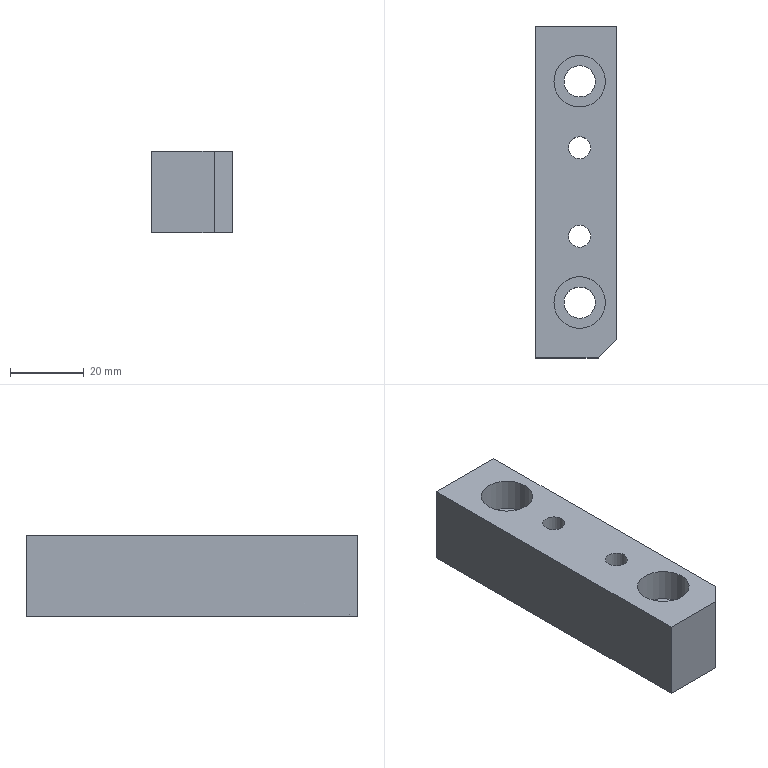Part | STEP file | P011002S004-003 | 1 solid | 15 faces | box 22 x 90 x 22 mm | volume 37795 mm3 | plane 9 | cylinder 6 | commonest cylinder face diameters 6 x2 8.5 x2 14 x2
STEP:
#1=CARTESIAN_POINT('',(0.,0.,0.));
#2=DIRECTION('',(0.,0.,1.));
#3=DIRECTION('',(1.,0.,0.));
#4=AXIS2_PLACEMENT_3D('',#1,#2,#3);
#5=CARTESIAN_POINT('',(90.,-233.,-3.));
#6=VERTEX_POINT('',#5);
#7=CARTESIAN_POINT('',(87.,-233.,-3.));
#8=DIRECTION('',(0.,0.,-1.));
#9=DIRECTION('',(1.,0.,0.));
#10=AXIS2_PLACEMENT_3D('',#7,#8,#9);
#11=CIRCLE('',#10,3.);
#12=CARTESIAN_POINT('',(75.,-258.,-3.));
#13=DIRECTION('',(0.,0.,-1.));
#14=DIRECTION('',(0.,1.,0.));
#15=AXIS2_PLACEMENT_3D('',#12,#13,#14);
#16=PLANE('',#15);
#17=CARTESIAN_POINT('',(25.,12.));
#18=DIRECTION('',(0.,1.));
#19=AXIS2_PLACEMENT_2D('',#17,#18);
#20=CIRCLE('',#19,3.);
#21=(GEOMETRIC_REPRESENTATION_CONTEXT(2)PARAMETRIC_REPRESENTATION_CONTEXT()REPRESENTATION_CONTEXT('',''));
#22=DEFINITIONAL_REPRESENTATION('',(#20),#21);
#23=PCURVE('',#16,#22);
#24=CARTESIAN_POINT('',(87.,-233.,19.));
#25=DIRECTION('',(0.,0.,-1.));
#26=DIRECTION('',(1.,0.,0.));
#27=AXIS2_PLACEMENT_3D('',#24,#25,#26);
#28=CYLINDRICAL_SURFACE('',#27,3.);
#29=CARTESIAN_POINT('',(0.,22.));
#30=DIRECTION('',(1.,0.));
#31=VECTOR('',#30,1.);
#32=LINE('',#29,#31);
#33=(GEOMETRIC_REPRESENTATION_CONTEXT(2)PARAMETRIC_REPRESENTATION_CONTEXT()REPRESENTATION_CONTEXT('',''));
#34=DEFINITIONAL_REPRESENTATION('',(#32),#33);
#35=PCURVE('',#28,#34);
#36=SURFACE_CURVE('',#11,(#23,#35),.PCURVE_S1.);
#37=EDGE_CURVE('',#6,#6,#36,.T.);
#38=ORIENTED_EDGE('',*,*,#37,.F.);
#39=EDGE_LOOP('',(#38));
#40=FACE_BOUND('',#39,.T.);
#41=CARTESIAN_POINT('',(90.,-257.,-3.));
#42=VERTEX_POINT('',#41);
#43=CARTESIAN_POINT('',(87.,-257.,-3.));
#44=DIRECTION('',(0.,0.,-1.));
#45=DIRECTION('',(1.,0.,0.));
#46=AXIS2_PLACEMENT_3D('',#43,#44,#45);
#47=CIRCLE('',#46,3.);
#48=CARTESIAN_POINT('',(1.,12.));
#49=DIRECTION('',(0.,1.));
#50=AXIS2_PLACEMENT_2D('',#48,#49);
#51=CIRCLE('',#50,3.);
#52=(GEOMETRIC_REPRESENTATION_CONTEXT(2)PARAMETRIC_REPRESENTATION_CONTEXT()REPRESENTATION_CONTEXT('',''));
#53=DEFINITIONAL_REPRESENTATION('',(#51),#52);
#54=PCURVE('',#16,#53);
#55=CARTESIAN_POINT('',(87.,-257.,19.));
#56=DIRECTION('',(0.,0.,-1.));
#57=DIRECTION('',(1.,0.,0.));
#58=AXIS2_PLACEMENT_3D('',#55,#56,#57);
#59=CYLINDRICAL_SURFACE('',#58,3.);
#60=CARTESIAN_POINT('',(0.,22.));
#61=DIRECTION('',(1.,0.));
#62=VECTOR('',#61,1.);
#63=LINE('',#60,#62);
#64=(GEOMETRIC_REPRESENTATION_CONTEXT(2)PARAMETRIC_REPRESENTATION_CONTEXT()REPRESENTATION_CONTEXT('',''));
#65=DEFINITIONAL_REPRESENTATION('',(#63),#64);
#66=PCURVE('',#59,#65);
#67=SURFACE_CURVE('',#47,(#54,#66),.PCURVE_S1.);
#68=EDGE_CURVE('',#42,#42,#67,.T.);
#69=ORIENTED_EDGE('',*,*,#68,.F.);
#70=EDGE_LOOP('',(#69));
#71=FACE_BOUND('',#70,.T.);
#72=CARTESIAN_POINT('',(75.,-290.,-3.));
#73=VERTEX_POINT('',#72);
#74=CARTESIAN_POINT('',(92.,-290.,-3.));
#75=VERTEX_POINT('',#74);
#76=CARTESIAN_POINT('',(75.,-290.,-3.));
#77=DIRECTION('',(1.,0.,0.));
#78=VECTOR('',#77,1.);
#79=LINE('',#76,#78);
#80=CARTESIAN_POINT('',(-32.,0.));
#81=DIRECTION('',(0.,1.));
#82=VECTOR('',#81,1.);
#83=LINE('',#80,#82);
#84=(GEOMETRIC_REPRESENTATION_CONTEXT(2)PARAMETRIC_REPRESENTATION_CONTEXT()REPRESENTATION_CONTEXT('',''));
#85=DEFINITIONAL_REPRESENTATION('',(#83),#84);
#86=PCURVE('',#16,#85);
#87=CARTESIAN_POINT('',(-325.,-290.,260.));
#88=DIRECTION('',(0.,1.,0.));
#89=DIRECTION('',(0.,0.,1.));
#90=AXIS2_PLACEMENT_3D('',#87,#88,#89);
#91=PLANE('',#90);
#92=CARTESIAN_POINT('',(-263.,400.));
#93=DIRECTION('',(0.,1.));
#94=VECTOR('',#93,1.);
#95=LINE('',#92,#94);
#96=(GEOMETRIC_REPRESENTATION_CONTEXT(2)PARAMETRIC_REPRESENTATION_CONTEXT()REPRESENTATION_CONTEXT('',''));
#97=DEFINITIONAL_REPRESENTATION('',(#95),#96);
#98=PCURVE('',#91,#97);
#99=SURFACE_CURVE('',#79,(#86,#98),.PCURVE_S1.);
#100=EDGE_CURVE('',#73,#75,#99,.T.);
#101=ORIENTED_EDGE('',*,*,#100,.F.);
#102=CARTESIAN_POINT('',(75.,-200.,-3.));
#103=VERTEX_POINT('',#102);
#104=CARTESIAN_POINT('',(75.,-258.,-3.));
#105=DIRECTION('',(0.,1.,0.));
#106=VECTOR('',#105,1.);
#107=LINE('',#104,#106);
#108=CARTESIAN_POINT('',(0.,0.));
#109=DIRECTION('',(1.,0.));
#110=VECTOR('',#109,1.);
#111=LINE('',#108,#110);
#112=(GEOMETRIC_REPRESENTATION_CONTEXT(2)PARAMETRIC_REPRESENTATION_CONTEXT()REPRESENTATION_CONTEXT('',''));
#113=DEFINITIONAL_REPRESENTATION('',(#111),#112);
#114=PCURVE('',#16,#113);
#115=CARTESIAN_POINT('',(75.,-258.,19.));
#116=DIRECTION('',(-1.,0.,0.));
#117=DIRECTION('',(0.,0.,-1.));
#118=AXIS2_PLACEMENT_3D('',#115,#116,#117);
#119=PLANE('',#118);
#120=CARTESIAN_POINT('',(22.,0.));
#121=DIRECTION('',(0.,-1.));
#122=VECTOR('',#121,1.);
#123=LINE('',#120,#122);
#124=(GEOMETRIC_REPRESENTATION_CONTEXT(2)PARAMETRIC_REPRESENTATION_CONTEXT()REPRESENTATION_CONTEXT('',''));
#125=DEFINITIONAL_REPRESENTATION('',(#123),#124);
#126=PCURVE('',#119,#125);
#127=SURFACE_CURVE('',#107,(#114,#126),.PCURVE_S1.);
#128=EDGE_CURVE('',#73,#103,#127,.T.);
#129=ORIENTED_EDGE('',*,*,#128,.T.);
#130=CARTESIAN_POINT('',(97.,-200.,-3.));
#131=VERTEX_POINT('',#130);
#132=CARTESIAN_POINT('',(-165.,-200.,-3.));
#133=DIRECTION('',(1.,0.,0.));
#134=VECTOR('',#133,1.);
#135=LINE('',#132,#134);
#136=CARTESIAN_POINT('',(58.,-240.));
#137=DIRECTION('',(0.,1.));
#138=VECTOR('',#137,1.);
#139=LINE('',#136,#138);
#140=(GEOMETRIC_REPRESENTATION_CONTEXT(2)PARAMETRIC_REPRESENTATION_CONTEXT()REPRESENTATION_CONTEXT('',''));
#141=DEFINITIONAL_REPRESENTATION('',(#139),#140);
#142=PCURVE('',#16,#141);
#143=CARTESIAN_POINT('',(-165.,-200.,-50.));
#144=DIRECTION('',(0.,-1.,0.));
#145=DIRECTION('',(0.,0.,1.));
#146=AXIS2_PLACEMENT_3D('',#143,#144,#145);
#147=PLANE('',#146);
#148=CARTESIAN_POINT('',(47.,0.));
#149=DIRECTION('',(0.,-1.));
#150=VECTOR('',#149,1.);
#151=LINE('',#148,#150);
#152=(GEOMETRIC_REPRESENTATION_CONTEXT(2)PARAMETRIC_REPRESENTATION_CONTEXT()REPRESENTATION_CONTEXT('',''));
#153=DEFINITIONAL_REPRESENTATION('',(#151),#152);
#154=PCURVE('',#147,#153);
#155=SURFACE_CURVE('',#135,(#142,#154),.PCURVE_S1.);
#156=EDGE_CURVE('',#103,#131,#155,.T.);
#157=ORIENTED_EDGE('',*,*,#156,.T.);
#158=CARTESIAN_POINT('',(97.,-285.,-3.));
#159=VERTEX_POINT('',#158);
#160=CARTESIAN_POINT('',(97.,-258.,-3.));
#161=DIRECTION('',(0.,1.,0.));
#162=VECTOR('',#161,1.);
#163=LINE('',#160,#162);
#164=CARTESIAN_POINT('',(0.,22.));
#165=DIRECTION('',(1.,0.));
#166=VECTOR('',#165,1.);
#167=LINE('',#164,#166);
#168=(GEOMETRIC_REPRESENTATION_CONTEXT(2)PARAMETRIC_REPRESENTATION_CONTEXT()REPRESENTATION_CONTEXT('',''));
#169=DEFINITIONAL_REPRESENTATION('',(#167),#168);
#170=PCURVE('',#16,#169);
#171=CARTESIAN_POINT('',(97.,-258.,19.));
#172=DIRECTION('',(-1.,0.,0.));
#173=DIRECTION('',(0.,0.,-1.));
#174=AXIS2_PLACEMENT_3D('',#171,#172,#173);
#175=PLANE('',#174);
#176=CARTESIAN_POINT('',(22.,0.));
#177=DIRECTION('',(0.,-1.));
#178=VECTOR('',#177,1.);
#179=LINE('',#176,#178);
#180=(GEOMETRIC_REPRESENTATION_CONTEXT(2)PARAMETRIC_REPRESENTATION_CONTEXT()REPRESENTATION_CONTEXT('',''));
#181=DEFINITIONAL_REPRESENTATION('',(#179),#180);
#182=PCURVE('',#175,#181);
#183=SURFACE_CURVE('',#163,(#170,#182),.PCURVE_S1.);
#184=EDGE_CURVE('',#159,#131,#183,.T.);
#185=ORIENTED_EDGE('',*,*,#184,.F.);
#186=CARTESIAN_POINT('',(99.5,-282.5,-3.));
#187=DIRECTION('',(0.7071,0.7071,0.));
#188=VECTOR('',#187,1.);
#189=LINE('',#186,#188);
#190=CARTESIAN_POINT('',(-24.5,24.5));
#191=DIRECTION('',(0.7071,0.7071));
#192=VECTOR('',#191,1.);
#193=LINE('',#190,#192);
#194=(GEOMETRIC_REPRESENTATION_CONTEXT(2)PARAMETRIC_REPRESENTATION_CONTEXT()REPRESENTATION_CONTEXT('',''));
#195=DEFINITIONAL_REPRESENTATION('',(#193),#194);
#196=PCURVE('',#16,#195);
#197=CARTESIAN_POINT('',(97.,-285.,19.));
#198=DIRECTION('',(-0.7071,0.7071,0.));
#199=DIRECTION('',(0.7071,0.7071,0.));
#200=AXIS2_PLACEMENT_3D('',#197,#198,#199);
#201=PLANE('',#200);
#202=CARTESIAN_POINT('',(3.536,22.));
#203=DIRECTION('',(1.,0.));
#204=VECTOR('',#203,1.);
#205=LINE('',#202,#204);
#206=(GEOMETRIC_REPRESENTATION_CONTEXT(2)PARAMETRIC_REPRESENTATION_CONTEXT()REPRESENTATION_CONTEXT('',''));
#207=DEFINITIONAL_REPRESENTATION('',(#205),#206);
#208=PCURVE('',#201,#207);
#209=SURFACE_CURVE('',#189,(#196,#208),.PCURVE_S1.);
#210=EDGE_CURVE('',#75,#159,#209,.T.);
#211=ORIENTED_EDGE('',*,*,#210,.F.);
#212=EDGE_LOOP('',(#101,#129,#157,#185,#211));
#213=FACE_BOUND('',#212,.T.);
#214=CARTESIAN_POINT('',(91.25,-215.,-3.));
#215=VERTEX_POINT('',#214);
#216=CARTESIAN_POINT('',(87.,-215.,-3.));
#217=DIRECTION('',(0.,0.,-1.));
#218=DIRECTION('',(1.,0.,0.));
#219=AXIS2_PLACEMENT_3D('',#216,#217,#218);
#220=CIRCLE('',#219,4.25);
#221=CARTESIAN_POINT('',(43.,12.));
#222=DIRECTION('',(0.,1.));
#223=AXIS2_PLACEMENT_2D('',#221,#222);
#224=CIRCLE('',#223,4.25);
#225=(GEOMETRIC_REPRESENTATION_CONTEXT(2)PARAMETRIC_REPRESENTATION_CONTEXT()REPRESENTATION_CONTEXT('',''));
#226=DEFINITIONAL_REPRESENTATION('',(#224),#225);
#227=PCURVE('',#16,#226);
#228=CARTESIAN_POINT('',(87.,-215.,19.));
#229=DIRECTION('',(0.,0.,-1.));
#230=DIRECTION('',(1.,0.,0.));
#231=AXIS2_PLACEMENT_3D('',#228,#229,#230);
#232=CYLINDRICAL_SURFACE('',#231,4.25);
#233=CARTESIAN_POINT('',(0.,22.));
#234=DIRECTION('',(1.,0.));
#235=VECTOR('',#234,1.);
#236=LINE('',#233,#235);
#237=(GEOMETRIC_REPRESENTATION_CONTEXT(2)PARAMETRIC_REPRESENTATION_CONTEXT()REPRESENTATION_CONTEXT('',''));
#238=DEFINITIONAL_REPRESENTATION('',(#236),#237);
#239=PCURVE('',#232,#238);
#240=SURFACE_CURVE('',#220,(#227,#239),.PCURVE_S1.);
#241=EDGE_CURVE('',#215,#215,#240,.T.);
#242=ORIENTED_EDGE('',*,*,#241,.F.);
#243=EDGE_LOOP('',(#242));
#244=FACE_BOUND('',#243,.T.);
#245=CARTESIAN_POINT('',(91.25,-275.,-3.));
#246=VERTEX_POINT('',#245);
#247=CARTESIAN_POINT('',(87.,-275.,-3.));
#248=DIRECTION('',(0.,0.,-1.));
#249=DIRECTION('',(1.,0.,0.));
#250=AXIS2_PLACEMENT_3D('',#247,#248,#249);
#251=CIRCLE('',#250,4.25);
#252=CARTESIAN_POINT('',(-17.,12.));
#253=DIRECTION('',(0.,1.));
#254=AXIS2_PLACEMENT_2D('',#252,#253);
#255=CIRCLE('',#254,4.25);
#256=(GEOMETRIC_REPRESENTATION_CONTEXT(2)PARAMETRIC_REPRESENTATION_CONTEXT()REPRESENTATION_CONTEXT('',''));
#257=DEFINITIONAL_REPRESENTATION('',(#255),#256);
#258=PCURVE('',#16,#257);
#259=CARTESIAN_POINT('',(87.,-275.,19.));
#260=DIRECTION('',(0.,0.,-1.));
#261=DIRECTION('',(1.,0.,0.));
#262=AXIS2_PLACEMENT_3D('',#259,#260,#261);
#263=CYLINDRICAL_SURFACE('',#262,4.25);
#264=CARTESIAN_POINT('',(0.,22.));
#265=DIRECTION('',(1.,0.));
#266=VECTOR('',#265,1.);
#267=LINE('',#264,#266);
#268=(GEOMETRIC_REPRESENTATION_CONTEXT(2)PARAMETRIC_REPRESENTATION_CONTEXT()REPRESENTATION_CONTEXT('',''));
#269=DEFINITIONAL_REPRESENTATION('',(#267),#268);
#270=PCURVE('',#263,#269);
#271=SURFACE_CURVE('',#251,(#258,#270),.PCURVE_S1.);
#272=EDGE_CURVE('',#246,#246,#271,.T.);
#273=ORIENTED_EDGE('',*,*,#272,.F.);
#274=EDGE_LOOP('',(#273));
#275=FACE_BOUND('',#274,.T.);
#276=ADVANCED_FACE('',(#40,#71,#213,#244,#275),#16,.T.);
#277=CARTESIAN_POINT('',(75.,-290.,19.));
#278=VERTEX_POINT('',#277);
#279=CARTESIAN_POINT('',(92.,-290.,19.));
#280=VERTEX_POINT('',#279);
#281=CARTESIAN_POINT('',(-325.,-290.,19.));
#282=DIRECTION('',(1.,0.,0.));
#283=VECTOR('',#282,1.);
#284=LINE('',#281,#283);
#285=CARTESIAN_POINT('',(-241.,0.));
#286=DIRECTION('',(0.,1.));
#287=VECTOR('',#286,1.);
#288=LINE('',#285,#287);
#289=(GEOMETRIC_REPRESENTATION_CONTEXT(2)PARAMETRIC_REPRESENTATION_CONTEXT()REPRESENTATION_CONTEXT('',''));
#290=DEFINITIONAL_REPRESENTATION('',(#288),#289);
#291=PCURVE('',#91,#290);
#292=CARTESIAN_POINT('',(-275.,-325.,19.));
#293=DIRECTION('',(0.,0.,1.));
#294=DIRECTION('',(-1.,0.,0.));
#295=AXIS2_PLACEMENT_3D('',#292,#293,#294);
#296=PLANE('',#295);
#297=CARTESIAN_POINT('',(50.,-35.));
#298=DIRECTION('',(-1.,0.));
#299=VECTOR('',#298,1.);
#300=LINE('',#297,#299);
#301=(GEOMETRIC_REPRESENTATION_CONTEXT(2)PARAMETRIC_REPRESENTATION_CONTEXT()REPRESENTATION_CONTEXT('',''));
#302=DEFINITIONAL_REPRESENTATION('',(#300),#301);
#303=PCURVE('',#296,#302);
#304=SURFACE_CURVE('',#284,(#291,#303),.PCURVE_S1.);
#305=EDGE_CURVE('',#278,#280,#304,.T.);
#306=ORIENTED_EDGE('',*,*,#305,.F.);
#307=CARTESIAN_POINT('',(75.,-290.,260.));
#308=DIRECTION('',(0.,0.,1.));
#309=VECTOR('',#308,1.);
#310=LINE('',#307,#309);
#311=CARTESIAN_POINT('',(0.,400.));
#312=DIRECTION('',(1.,0.));
#313=VECTOR('',#312,1.);
#314=LINE('',#311,#313);
#315=(GEOMETRIC_REPRESENTATION_CONTEXT(2)PARAMETRIC_REPRESENTATION_CONTEXT()REPRESENTATION_CONTEXT('',''));
#316=DEFINITIONAL_REPRESENTATION('',(#314),#315);
#317=PCURVE('',#91,#316);
#318=CARTESIAN_POINT('',(-241.,32.));
#319=DIRECTION('',(-1.,0.));
#320=VECTOR('',#319,1.);
#321=LINE('',#318,#320);
#322=(GEOMETRIC_REPRESENTATION_CONTEXT(2)PARAMETRIC_REPRESENTATION_CONTEXT()REPRESENTATION_CONTEXT('',''));
#323=DEFINITIONAL_REPRESENTATION('',(#321),#322);
#324=PCURVE('',#119,#323);
#325=SURFACE_CURVE('',#310,(#317,#324),.PCURVE_S1.);
#326=EDGE_CURVE('',#73,#278,#325,.T.);
#327=ORIENTED_EDGE('',*,*,#326,.F.);
#328=ORIENTED_EDGE('',*,*,#100,.T.);
#329=CARTESIAN_POINT('',(92.,-290.,-3.));
#330=DIRECTION('',(0.,0.,-1.));
#331=VECTOR('',#330,1.);
#332=LINE('',#329,#331);
#333=CARTESIAN_POINT('',(-263.,417.));
#334=DIRECTION('',(-1.,0.));
#335=VECTOR('',#334,1.);
#336=LINE('',#333,#335);
#337=(GEOMETRIC_REPRESENTATION_CONTEXT(2)PARAMETRIC_REPRESENTATION_CONTEXT()REPRESENTATION_CONTEXT('',''));
#338=DEFINITIONAL_REPRESENTATION('',(#336),#337);
#339=PCURVE('',#91,#338);
#340=CARTESIAN_POINT('',(-7.071,22.));
#341=DIRECTION('',(0.,1.));
#342=VECTOR('',#341,1.);
#343=LINE('',#340,#342);
#344=(GEOMETRIC_REPRESENTATION_CONTEXT(2)PARAMETRIC_REPRESENTATION_CONTEXT()REPRESENTATION_CONTEXT('',''));
#345=DEFINITIONAL_REPRESENTATION('',(#343),#344);
#346=PCURVE('',#201,#345);
#347=SURFACE_CURVE('',#332,(#339,#346),.PCURVE_S1.);
#348=EDGE_CURVE('',#280,#75,#347,.T.);
#349=ORIENTED_EDGE('',*,*,#348,.F.);
#350=EDGE_LOOP('',(#306,#327,#328,#349));
#351=FACE_BOUND('',#350,.T.);
#352=ADVANCED_FACE('',(#351),#91,.F.);
#353=CARTESIAN_POINT('',(80.,-275.,19.));
#354=VERTEX_POINT('',#353);
#355=CARTESIAN_POINT('',(87.,-275.,19.));
#356=DIRECTION('',(0.,0.,-1.));
#357=DIRECTION('',(-1.,0.,0.));
#358=AXIS2_PLACEMENT_3D('',#355,#356,#357);
#359=CIRCLE('',#358,7.);
#360=CARTESIAN_POINT('',(-355.,-50.));
#361=CARTESIAN_POINT('',(-355.,-62.124));
#362=CARTESIAN_POINT('',(-365.5,-56.062));
#363=CARTESIAN_POINT('',(-376.,-50.));
#364=CARTESIAN_POINT('',(-365.5,-43.938));
#365=CARTESIAN_POINT('',(-355.,-37.876));
#366=CARTESIAN_POINT('',(-355.,-50.));
#367=(BOUNDED_CURVE()B_SPLINE_CURVE(2,(#360,#361,#362,#363,#364,#365,#366),.UNSPECIFIED.,.T.,.F.)B_SPLINE_CURVE_WITH_KNOTS((1,2,2,2,2,1),(-2.094,0.,2.094,4.189,6.283,8.378),.UNSPECIFIED.)CURVE()GEOMETRIC_REPRESENTATION_ITEM()RATIONAL_B_SPLINE_CURVE((1.,0.5,1.,0.5,1.,0.5,1.))REPRESENTATION_ITEM(''));
#368=(GEOMETRIC_REPRESENTATION_CONTEXT(2)PARAMETRIC_REPRESENTATION_CONTEXT()REPRESENTATION_CONTEXT('',''));
#369=DEFINITIONAL_REPRESENTATION('',(#367),#368);
#370=PCURVE('',#296,#369);
#371=CARTESIAN_POINT('',(87.,-275.,19.));
#372=DIRECTION('',(0.,0.,-1.));
#373=DIRECTION('',(1.,0.,0.));
#374=AXIS2_PLACEMENT_3D('',#371,#372,#373);
#375=CYLINDRICAL_SURFACE('',#374,7.);
#376=CARTESIAN_POINT('',(3.142,0.));
#377=DIRECTION('',(1.,0.));
#378=VECTOR('',#377,1.);
#379=LINE('',#376,#378);
#380=(GEOMETRIC_REPRESENTATION_CONTEXT(2)PARAMETRIC_REPRESENTATION_CONTEXT()REPRESENTATION_CONTEXT('',''));
#381=DEFINITIONAL_REPRESENTATION('',(#379),#380);
#382=PCURVE('',#375,#381);
#383=SURFACE_CURVE('',#359,(#370,#382),.PCURVE_S1.);
#384=EDGE_CURVE('',#354,#354,#383,.T.);
#385=ORIENTED_EDGE('',*,*,#384,.T.);
#386=EDGE_LOOP('',(#385));
#387=FACE_BOUND('',#386,.T.);
#388=CARTESIAN_POINT('',(84.,-233.,19.));
#389=VERTEX_POINT('',#388);
#390=CARTESIAN_POINT('',(90.,-233.,19.));
#391=VERTEX_POINT('',#390);
#392=CARTESIAN_POINT('',(87.,-233.,19.));
#393=DIRECTION('',(0.,0.,-1.));
#394=DIRECTION('',(-1.,0.,0.));
#395=AXIS2_PLACEMENT_3D('',#392,#393,#394);
#396=CIRCLE('',#395,3.);
#397=CARTESIAN_POINT('',(-359.,-92.));
#398=CARTESIAN_POINT('',(-359.,-97.196));
#399=CARTESIAN_POINT('',(-363.5,-94.598));
#400=CARTESIAN_POINT('',(-368.,-92.));
#401=CARTESIAN_POINT('',(-363.5,-89.402));
#402=CARTESIAN_POINT('',(-359.,-86.804));
#403=CARTESIAN_POINT('',(-359.,-92.));
#404=(BOUNDED_CURVE()B_SPLINE_CURVE(2,(#397,#398,#399,#400,#401,#402,#403),.UNSPECIFIED.,.T.,.F.)B_SPLINE_CURVE_WITH_KNOTS((1,2,2,2,2,1),(-2.094,0.,2.094,4.189,6.283,8.378),.UNSPECIFIED.)CURVE()GEOMETRIC_REPRESENTATION_ITEM()RATIONAL_B_SPLINE_CURVE((1.,0.5,1.,0.5,1.,0.5,1.))REPRESENTATION_ITEM(''));
#405=(GEOMETRIC_REPRESENTATION_CONTEXT(2)PARAMETRIC_REPRESENTATION_CONTEXT()REPRESENTATION_CONTEXT('',''));
#406=DEFINITIONAL_REPRESENTATION('',(#404),#405);
#407=PCURVE('',#296,#406);
#408=CARTESIAN_POINT('',(3.142,0.));
#409=DIRECTION('',(1.,0.));
#410=VECTOR('',#409,1.);
#411=LINE('',#408,#410);
#412=(GEOMETRIC_REPRESENTATION_CONTEXT(2)PARAMETRIC_REPRESENTATION_CONTEXT()REPRESENTATION_CONTEXT('',''));
#413=DEFINITIONAL_REPRESENTATION('',(#411),#412);
#414=PCURVE('',#28,#413);
#415=SURFACE_CURVE('',#396,(#407,#414),.PCURVE_S1.);
#416=EDGE_CURVE('',#389,#391,#415,.T.);
#417=ORIENTED_EDGE('',*,*,#416,.T.);
#418=CARTESIAN_POINT('',(87.,-233.,19.));
#419=DIRECTION('',(0.,0.,-1.));
#420=DIRECTION('',(-1.,0.,0.));
#421=AXIS2_PLACEMENT_3D('',#418,#419,#420);
#422=CIRCLE('',#421,3.);
#423=CARTESIAN_POINT('',(-359.,-92.));
#424=CARTESIAN_POINT('',(-359.,-97.196));
#425=CARTESIAN_POINT('',(-363.5,-94.598));
#426=CARTESIAN_POINT('',(-368.,-92.));
#427=CARTESIAN_POINT('',(-363.5,-89.402));
#428=CARTESIAN_POINT('',(-359.,-86.804));
#429=CARTESIAN_POINT('',(-359.,-92.));
#430=(BOUNDED_CURVE()B_SPLINE_CURVE(2,(#423,#424,#425,#426,#427,#428,#429),.UNSPECIFIED.,.T.,.F.)B_SPLINE_CURVE_WITH_KNOTS((1,2,2,2,2,1),(-2.094,0.,2.094,4.189,6.283,8.378),.UNSPECIFIED.)CURVE()GEOMETRIC_REPRESENTATION_ITEM()RATIONAL_B_SPLINE_CURVE((1.,0.5,1.,0.5,1.,0.5,1.))REPRESENTATION_ITEM(''));
#431=(GEOMETRIC_REPRESENTATION_CONTEXT(2)PARAMETRIC_REPRESENTATION_CONTEXT()REPRESENTATION_CONTEXT('',''));
#432=DEFINITIONAL_REPRESENTATION('',(#430),#431);
#433=PCURVE('',#296,#432);
#434=CARTESIAN_POINT('',(-3.142,0.));
#435=DIRECTION('',(1.,0.));
#436=VECTOR('',#435,1.);
#437=LINE('',#434,#436);
#438=(GEOMETRIC_REPRESENTATION_CONTEXT(2)PARAMETRIC_REPRESENTATION_CONTEXT()REPRESENTATION_CONTEXT('',''));
#439=DEFINITIONAL_REPRESENTATION('',(#437),#438);
#440=PCURVE('',#28,#439);
#441=SURFACE_CURVE('',#422,(#433,#440),.PCURVE_S1.);
#442=EDGE_CURVE('',#391,#389,#441,.T.);
#443=ORIENTED_EDGE('',*,*,#442,.T.);
#444=EDGE_LOOP('',(#417,#443));
#445=FACE_BOUND('',#444,.T.);
#446=CARTESIAN_POINT('',(80.,-215.,19.));
#447=VERTEX_POINT('',#446);
#448=CARTESIAN_POINT('',(87.,-215.,19.));
#449=DIRECTION('',(0.,0.,-1.));
#450=DIRECTION('',(-1.,0.,0.));
#451=AXIS2_PLACEMENT_3D('',#448,#449,#450);
#452=CIRCLE('',#451,7.);
#453=CARTESIAN_POINT('',(-355.,-110.));
#454=CARTESIAN_POINT('',(-355.,-122.124));
#455=CARTESIAN_POINT('',(-365.5,-116.062));
#456=CARTESIAN_POINT('',(-376.,-110.));
#457=CARTESIAN_POINT('',(-365.5,-103.938));
#458=CARTESIAN_POINT('',(-355.,-97.876));
#459=CARTESIAN_POINT('',(-355.,-110.));
#460=(BOUNDED_CURVE()B_SPLINE_CURVE(2,(#453,#454,#455,#456,#457,#458,#459),.UNSPECIFIED.,.T.,.F.)B_SPLINE_CURVE_WITH_KNOTS((1,2,2,2,2,1),(-2.094,0.,2.094,4.189,6.283,8.378),.UNSPECIFIED.)CURVE()GEOMETRIC_REPRESENTATION_ITEM()RATIONAL_B_SPLINE_CURVE((1.,0.5,1.,0.5,1.,0.5,1.))REPRESENTATION_ITEM(''));
#461=(GEOMETRIC_REPRESENTATION_CONTEXT(2)PARAMETRIC_REPRESENTATION_CONTEXT()REPRESENTATION_CONTEXT('',''));
#462=DEFINITIONAL_REPRESENTATION('',(#460),#461);
#463=PCURVE('',#296,#462);
#464=CARTESIAN_POINT('',(87.,-215.,19.));
#465=DIRECTION('',(0.,0.,-1.));
#466=DIRECTION('',(1.,0.,0.));
#467=AXIS2_PLACEMENT_3D('',#464,#465,#466);
#468=CYLINDRICAL_SURFACE('',#467,7.);
#469=CARTESIAN_POINT('',(3.142,0.));
#470=DIRECTION('',(1.,0.));
#471=VECTOR('',#470,1.);
#472=LINE('',#469,#471);
#473=(GEOMETRIC_REPRESENTATION_CONTEXT(2)PARAMETRIC_REPRESENTATION_CONTEXT()REPRESENTATION_CONTEXT('',''));
#474=DEFINITIONAL_REPRESENTATION('',(#472),#473);
#475=PCURVE('',#468,#474);
#476=SURFACE_CURVE('',#452,(#463,#475),.PCURVE_S1.);
#477=EDGE_CURVE('',#447,#447,#476,.T.);
#478=ORIENTED_EDGE('',*,*,#477,.T.);
#479=EDGE_LOOP('',(#478));
#480=FACE_BOUND('',#479,.T.);
#481=CARTESIAN_POINT('',(84.,-257.,19.));
#482=VERTEX_POINT('',#481);
#483=CARTESIAN_POINT('',(90.,-257.,19.));
#484=VERTEX_POINT('',#483);
#485=CARTESIAN_POINT('',(87.,-257.,19.));
#486=DIRECTION('',(0.,0.,-1.));
#487=DIRECTION('',(-1.,0.,0.));
#488=AXIS2_PLACEMENT_3D('',#485,#486,#487);
#489=CIRCLE('',#488,3.);
#490=CARTESIAN_POINT('',(-359.,-68.));
#491=CARTESIAN_POINT('',(-359.,-73.196));
#492=CARTESIAN_POINT('',(-363.5,-70.598));
#493=CARTESIAN_POINT('',(-368.,-68.));
#494=CARTESIAN_POINT('',(-363.5,-65.402));
#495=CARTESIAN_POINT('',(-359.,-62.804));
#496=CARTESIAN_POINT('',(-359.,-68.));
#497=(BOUNDED_CURVE()B_SPLINE_CURVE(2,(#490,#491,#492,#493,#494,#495,#496),.UNSPECIFIED.,.T.,.F.)B_SPLINE_CURVE_WITH_KNOTS((1,2,2,2,2,1),(-2.094,0.,2.094,4.189,6.283,8.378),.UNSPECIFIED.)CURVE()GEOMETRIC_REPRESENTATION_ITEM()RATIONAL_B_SPLINE_CURVE((1.,0.5,1.,0.5,1.,0.5,1.))REPRESENTATION_ITEM(''));
#498=(GEOMETRIC_REPRESENTATION_CONTEXT(2)PARAMETRIC_REPRESENTATION_CONTEXT()REPRESENTATION_CONTEXT('',''));
#499=DEFINITIONAL_REPRESENTATION('',(#497),#498);
#500=PCURVE('',#296,#499);
#501=CARTESIAN_POINT('',(3.142,0.));
#502=DIRECTION('',(1.,0.));
#503=VECTOR('',#502,1.);
#504=LINE('',#501,#503);
#505=(GEOMETRIC_REPRESENTATION_CONTEXT(2)PARAMETRIC_REPRESENTATION_CONTEXT()REPRESENTATION_CONTEXT('',''));
#506=DEFINITIONAL_REPRESENTATION('',(#504),#505);
#507=PCURVE('',#59,#506);
#508=SURFACE_CURVE('',#489,(#500,#507),.PCURVE_S1.);
#509=EDGE_CURVE('',#482,#484,#508,.T.);
#510=ORIENTED_EDGE('',*,*,#509,.T.);
#511=CARTESIAN_POINT('',(87.,-257.,19.));
#512=DIRECTION('',(0.,0.,-1.));
#513=DIRECTION('',(-1.,0.,0.));
#514=AXIS2_PLACEMENT_3D('',#511,#512,#513);
#515=CIRCLE('',#514,3.);
#516=CARTESIAN_POINT('',(-359.,-68.));
#517=CARTESIAN_POINT('',(-359.,-73.196));
#518=CARTESIAN_POINT('',(-363.5,-70.598));
#519=CARTESIAN_POINT('',(-368.,-68.));
#520=CARTESIAN_POINT('',(-363.5,-65.402));
#521=CARTESIAN_POINT('',(-359.,-62.804));
#522=CARTESIAN_POINT('',(-359.,-68.));
#523=(BOUNDED_CURVE()B_SPLINE_CURVE(2,(#516,#517,#518,#519,#520,#521,#522),.UNSPECIFIED.,.T.,.F.)B_SPLINE_CURVE_WITH_KNOTS((1,2,2,2,2,1),(-2.094,0.,2.094,4.189,6.283,8.378),.UNSPECIFIED.)CURVE()GEOMETRIC_REPRESENTATION_ITEM()RATIONAL_B_SPLINE_CURVE((1.,0.5,1.,0.5,1.,0.5,1.))REPRESENTATION_ITEM(''));
#524=(GEOMETRIC_REPRESENTATION_CONTEXT(2)PARAMETRIC_REPRESENTATION_CONTEXT()REPRESENTATION_CONTEXT('',''));
#525=DEFINITIONAL_REPRESENTATION('',(#523),#524);
#526=PCURVE('',#296,#525);
#527=CARTESIAN_POINT('',(-3.142,0.));
#528=DIRECTION('',(1.,0.));
#529=VECTOR('',#528,1.);
#530=LINE('',#527,#529);
#531=(GEOMETRIC_REPRESENTATION_CONTEXT(2)PARAMETRIC_REPRESENTATION_CONTEXT()REPRESENTATION_CONTEXT('',''));
#532=DEFINITIONAL_REPRESENTATION('',(#530),#531);
#533=PCURVE('',#59,#532);
#534=SURFACE_CURVE('',#515,(#526,#533),.PCURVE_S1.);
#535=EDGE_CURVE('',#484,#482,#534,.T.);
#536=ORIENTED_EDGE('',*,*,#535,.T.);
#537=EDGE_LOOP('',(#510,#536));
#538=FACE_BOUND('',#537,.T.);
#539=CARTESIAN_POINT('',(97.,-285.,19.));
#540=VERTEX_POINT('',#539);
#541=CARTESIAN_POINT('',(97.,-200.,19.));
#542=VERTEX_POINT('',#541);
#543=CARTESIAN_POINT('',(97.,-325.,19.));
#544=DIRECTION('',(0.,1.,0.));
#545=VECTOR('',#544,1.);
#546=LINE('',#543,#545);
#547=CARTESIAN_POINT('',(-372.,0.));
#548=DIRECTION('',(0.,-1.));
#549=VECTOR('',#548,1.);
#550=LINE('',#547,#549);
#551=(GEOMETRIC_REPRESENTATION_CONTEXT(2)PARAMETRIC_REPRESENTATION_CONTEXT()REPRESENTATION_CONTEXT('',''));
#552=DEFINITIONAL_REPRESENTATION('',(#550),#551);
#553=PCURVE('',#296,#552);
#554=CARTESIAN_POINT('',(0.,67.));
#555=DIRECTION('',(0.,-1.));
#556=VECTOR('',#555,1.);
#557=LINE('',#554,#556);
#558=(GEOMETRIC_REPRESENTATION_CONTEXT(2)PARAMETRIC_REPRESENTATION_CONTEXT()REPRESENTATION_CONTEXT('',''));
#559=DEFINITIONAL_REPRESENTATION('',(#557),#558);
#560=PCURVE('',#175,#559);
#561=SURFACE_CURVE('',#546,(#553,#560),.PCURVE_S1.);
#562=EDGE_CURVE('',#540,#542,#561,.T.);
#563=ORIENTED_EDGE('',*,*,#562,.T.);
#564=CARTESIAN_POINT('',(75.,-200.,19.));
#565=VERTEX_POINT('',#564);
#566=CARTESIAN_POINT('',(-275.,-200.,19.));
#567=DIRECTION('',(1.,0.,0.));
#568=VECTOR('',#567,1.);
#569=LINE('',#566,#568);
#570=CARTESIAN_POINT('',(0.,-125.));
#571=DIRECTION('',(-1.,0.));
#572=VECTOR('',#571,1.);
#573=LINE('',#570,#572);
#574=(GEOMETRIC_REPRESENTATION_CONTEXT(2)PARAMETRIC_REPRESENTATION_CONTEXT()REPRESENTATION_CONTEXT('',''));
#575=DEFINITIONAL_REPRESENTATION('',(#573),#574);
#576=PCURVE('',#296,#575);
#577=CARTESIAN_POINT('',(69.,110.));
#578=DIRECTION('',(0.,-1.));
#579=VECTOR('',#578,1.);
#580=LINE('',#577,#579);
#581=(GEOMETRIC_REPRESENTATION_CONTEXT(2)PARAMETRIC_REPRESENTATION_CONTEXT()REPRESENTATION_CONTEXT('',''));
#582=DEFINITIONAL_REPRESENTATION('',(#580),#581);
#583=PCURVE('',#147,#582);
#584=SURFACE_CURVE('',#569,(#576,#583),.PCURVE_S1.);
#585=EDGE_CURVE('',#565,#542,#584,.T.);
#586=ORIENTED_EDGE('',*,*,#585,.F.);
#587=CARTESIAN_POINT('',(75.,-325.,19.));
#588=DIRECTION('',(0.,1.,0.));
#589=VECTOR('',#588,1.);
#590=LINE('',#587,#589);
#591=CARTESIAN_POINT('',(-350.,0.));
#592=DIRECTION('',(0.,-1.));
#593=VECTOR('',#592,1.);
#594=LINE('',#591,#593);
#595=(GEOMETRIC_REPRESENTATION_CONTEXT(2)PARAMETRIC_REPRESENTATION_CONTEXT()REPRESENTATION_CONTEXT('',''));
#596=DEFINITIONAL_REPRESENTATION('',(#594),#595);
#597=PCURVE('',#296,#596);
#598=CARTESIAN_POINT('',(0.,67.));
#599=DIRECTION('',(0.,-1.));
#600=VECTOR('',#599,1.);
#601=LINE('',#598,#600);
#602=(GEOMETRIC_REPRESENTATION_CONTEXT(2)PARAMETRIC_REPRESENTATION_CONTEXT()REPRESENTATION_CONTEXT('',''));
#603=DEFINITIONAL_REPRESENTATION('',(#601),#602);
#604=PCURVE('',#119,#603);
#605=SURFACE_CURVE('',#590,(#597,#604),.PCURVE_S1.);
#606=EDGE_CURVE('',#278,#565,#605,.T.);
#607=ORIENTED_EDGE('',*,*,#606,.F.);
#608=ORIENTED_EDGE('',*,*,#305,.T.);
#609=CARTESIAN_POINT('',(-109.,-491.,19.));
#610=DIRECTION('',(-0.7071,-0.7071,0.));
#611=VECTOR('',#610,1.);
#612=LINE('',#609,#611);
#613=CARTESIAN_POINT('',(-166.,166.));
#614=DIRECTION('',(0.7071,0.7071));
#615=VECTOR('',#614,1.);
#616=LINE('',#613,#615);
#617=(GEOMETRIC_REPRESENTATION_CONTEXT(2)PARAMETRIC_REPRESENTATION_CONTEXT()REPRESENTATION_CONTEXT('',''));
#618=DEFINITIONAL_REPRESENTATION('',(#616),#617);
#619=PCURVE('',#296,#618);
#620=CARTESIAN_POINT('',(-291.328,0.));
#621=DIRECTION('',(-1.,0.));
#622=VECTOR('',#621,1.);
#623=LINE('',#620,#622);
#624=(GEOMETRIC_REPRESENTATION_CONTEXT(2)PARAMETRIC_REPRESENTATION_CONTEXT()REPRESENTATION_CONTEXT('',''));
#625=DEFINITIONAL_REPRESENTATION('',(#623),#624);
#626=PCURVE('',#201,#625);
#627=SURFACE_CURVE('',#612,(#619,#626),.PCURVE_S1.);
#628=EDGE_CURVE('',#540,#280,#627,.T.);
#629=ORIENTED_EDGE('',*,*,#628,.F.);
#630=EDGE_LOOP('',(#563,#586,#607,#608,#629));
#631=FACE_BOUND('',#630,.T.);
#632=ADVANCED_FACE('',(#387,#445,#480,#538,#631),#296,.T.);
#633=CARTESIAN_POINT('',(75.,-200.,19.));
#634=DIRECTION('',(0.,0.,1.));
#635=VECTOR('',#634,1.);
#636=LINE('',#633,#635);
#637=CARTESIAN_POINT('',(69.,-240.));
#638=DIRECTION('',(1.,0.));
#639=VECTOR('',#638,1.);
#640=LINE('',#637,#639);
#641=(GEOMETRIC_REPRESENTATION_CONTEXT(2)PARAMETRIC_REPRESENTATION_CONTEXT()REPRESENTATION_CONTEXT('',''));
#642=DEFINITIONAL_REPRESENTATION('',(#640),#641);
#643=PCURVE('',#147,#642);
#644=CARTESIAN_POINT('',(0.,-58.));
#645=DIRECTION('',(-1.,0.));
#646=VECTOR('',#645,1.);
#647=LINE('',#644,#646);
#648=(GEOMETRIC_REPRESENTATION_CONTEXT(2)PARAMETRIC_REPRESENTATION_CONTEXT()REPRESENTATION_CONTEXT('',''));
#649=DEFINITIONAL_REPRESENTATION('',(#647),#648);
#650=PCURVE('',#119,#649);
#651=SURFACE_CURVE('',#636,(#643,#650),.PCURVE_S1.);
#652=EDGE_CURVE('',#103,#565,#651,.T.);
#653=ORIENTED_EDGE('',*,*,#652,.T.);
#654=ORIENTED_EDGE('',*,*,#585,.T.);
#655=CARTESIAN_POINT('',(97.,-200.,19.));
#656=DIRECTION('',(0.,0.,1.));
#657=VECTOR('',#656,1.);
#658=LINE('',#655,#657);
#659=CARTESIAN_POINT('',(69.,-262.));
#660=DIRECTION('',(1.,0.));
#661=VECTOR('',#660,1.);
#662=LINE('',#659,#661);
#663=(GEOMETRIC_REPRESENTATION_CONTEXT(2)PARAMETRIC_REPRESENTATION_CONTEXT()REPRESENTATION_CONTEXT('',''));
#664=DEFINITIONAL_REPRESENTATION('',(#662),#663);
#665=PCURVE('',#147,#664);
#666=CARTESIAN_POINT('',(0.,-58.));
#667=DIRECTION('',(-1.,0.));
#668=VECTOR('',#667,1.);
#669=LINE('',#666,#668);
#670=(GEOMETRIC_REPRESENTATION_CONTEXT(2)PARAMETRIC_REPRESENTATION_CONTEXT()REPRESENTATION_CONTEXT('',''));
#671=DEFINITIONAL_REPRESENTATION('',(#669),#670);
#672=PCURVE('',#175,#671);
#673=SURFACE_CURVE('',#658,(#665,#672),.PCURVE_S1.);
#674=EDGE_CURVE('',#131,#542,#673,.T.);
#675=ORIENTED_EDGE('',*,*,#674,.F.);
#676=ORIENTED_EDGE('',*,*,#156,.F.);
#677=EDGE_LOOP('',(#653,#654,#675,#676));
#678=FACE_BOUND('',#677,.T.);
#679=ADVANCED_FACE('',(#678),#147,.F.);
#680=ORIENTED_EDGE('',*,*,#184,.T.);
#681=ORIENTED_EDGE('',*,*,#674,.T.);
#682=ORIENTED_EDGE('',*,*,#562,.F.);
#683=CARTESIAN_POINT('',(97.,-285.,19.));
#684=DIRECTION('',(0.,0.,1.));
#685=VECTOR('',#684,1.);
#686=LINE('',#683,#685);
#687=CARTESIAN_POINT('',(0.,27.));
#688=DIRECTION('',(-1.,0.));
#689=VECTOR('',#688,1.);
#690=LINE('',#687,#689);
#691=(GEOMETRIC_REPRESENTATION_CONTEXT(2)PARAMETRIC_REPRESENTATION_CONTEXT()REPRESENTATION_CONTEXT('',''));
#692=DEFINITIONAL_REPRESENTATION('',(#690),#691);
#693=PCURVE('',#175,#692);
#694=CARTESIAN_POINT('',(0.,0.));
#695=DIRECTION('',(0.,-1.));
#696=VECTOR('',#695,1.);
#697=LINE('',#694,#696);
#698=(GEOMETRIC_REPRESENTATION_CONTEXT(2)PARAMETRIC_REPRESENTATION_CONTEXT()REPRESENTATION_CONTEXT('',''));
#699=DEFINITIONAL_REPRESENTATION('',(#697),#698);
#700=PCURVE('',#201,#699);
#701=SURFACE_CURVE('',#686,(#693,#700),.PCURVE_S1.);
#702=EDGE_CURVE('',#159,#540,#701,.T.);
#703=ORIENTED_EDGE('',*,*,#702,.F.);
#704=EDGE_LOOP('',(#680,#681,#682,#703));
#705=FACE_BOUND('',#704,.T.);
#706=ADVANCED_FACE('',(#705),#175,.F.);
#707=ORIENTED_EDGE('',*,*,#606,.T.);
#708=ORIENTED_EDGE('',*,*,#652,.F.);
#709=ORIENTED_EDGE('',*,*,#128,.F.);
#710=ORIENTED_EDGE('',*,*,#326,.T.);
#711=EDGE_LOOP('',(#707,#708,#709,#710));
#712=FACE_BOUND('',#711,.T.);
#713=ADVANCED_FACE('',(#712),#119,.T.);
#714=ORIENTED_EDGE('',*,*,#210,.T.);
#715=ORIENTED_EDGE('',*,*,#702,.T.);
#716=ORIENTED_EDGE('',*,*,#628,.T.);
#717=ORIENTED_EDGE('',*,*,#348,.T.);
#718=EDGE_LOOP('',(#714,#715,#716,#717));
#719=FACE_BOUND('',#718,.T.);
#720=ADVANCED_FACE('',(#719),#201,.F.);
#721=ORIENTED_EDGE('',*,*,#68,.F.);
#722=CARTESIAN_POINT('',(90.,-257.,19.));
#723=CARTESIAN_POINT('',(90.,-257.,-3.));
#724=B_SPLINE_CURVE_WITH_KNOTS('',1,(#722,#723),.UNSPECIFIED.,.F.,.F.,(2,2),(0.,22.),.PIECEWISE_BEZIER_KNOTS.);
#725=CARTESIAN_POINT('',(0.,0.));
#726=DIRECTION('',(0.,1.));
#727=VECTOR('',#726,1.);
#728=LINE('',#725,#727);
#729=(GEOMETRIC_REPRESENTATION_CONTEXT(2)PARAMETRIC_REPRESENTATION_CONTEXT()REPRESENTATION_CONTEXT('',''));
#730=DEFINITIONAL_REPRESENTATION('',(#728),#729);
#731=PCURVE('',#59,#730);
#732=CARTESIAN_POINT('',(6.283,0.));
#733=DIRECTION('',(0.,1.));
#734=VECTOR('',#733,1.);
#735=LINE('',#732,#734);
#736=(GEOMETRIC_REPRESENTATION_CONTEXT(2)PARAMETRIC_REPRESENTATION_CONTEXT()REPRESENTATION_CONTEXT('',''));
#737=DEFINITIONAL_REPRESENTATION('',(#735),#736);
#738=PCURVE('',#59,#737);
#739=SEAM_CURVE('',#724,(#731,#738),.PCURVE_S1.);
#740=EDGE_CURVE('',#484,#42,#739,.T.);
#741=ORIENTED_EDGE('',*,*,#740,.F.);
#742=ORIENTED_EDGE('',*,*,#535,.T.);
#743=ORIENTED_EDGE('',*,*,#509,.T.);
#744=ORIENTED_EDGE('',*,*,#740,.T.);
#745=EDGE_LOOP('',(#721,#741,#742,#743,#744));
#746=FACE_BOUND('',#745,.F.);
#747=ADVANCED_FACE('',(#746),#59,.F.);
#748=ORIENTED_EDGE('',*,*,#241,.F.);
#749=CARTESIAN_POINT('',(91.25,-215.,10.));
#750=VERTEX_POINT('',#749);
#751=CARTESIAN_POINT('',(91.25,-215.,10.));
#752=CARTESIAN_POINT('',(91.25,-215.,-3.));
#753=B_SPLINE_CURVE_WITH_KNOTS('',1,(#751,#752),.UNSPECIFIED.,.F.,.F.,(2,2),(9.,22.),.PIECEWISE_BEZIER_KNOTS.);
#754=CARTESIAN_POINT('',(0.,0.));
#755=DIRECTION('',(0.,1.));
#756=VECTOR('',#755,1.);
#757=LINE('',#754,#756);
#758=(GEOMETRIC_REPRESENTATION_CONTEXT(2)PARAMETRIC_REPRESENTATION_CONTEXT()REPRESENTATION_CONTEXT('',''));
#759=DEFINITIONAL_REPRESENTATION('',(#757),#758);
#760=PCURVE('',#232,#759);
#761=CARTESIAN_POINT('',(6.283,0.));
#762=DIRECTION('',(0.,1.));
#763=VECTOR('',#762,1.);
#764=LINE('',#761,#763);
#765=(GEOMETRIC_REPRESENTATION_CONTEXT(2)PARAMETRIC_REPRESENTATION_CONTEXT()REPRESENTATION_CONTEXT('',''));
#766=DEFINITIONAL_REPRESENTATION('',(#764),#765);
#767=PCURVE('',#232,#766);
#768=SEAM_CURVE('',#753,(#760,#767),.PCURVE_S1.);
#769=EDGE_CURVE('',#750,#215,#768,.T.);
#770=ORIENTED_EDGE('',*,*,#769,.F.);
#771=CARTESIAN_POINT('',(82.75,-215.,10.));
#772=VERTEX_POINT('',#771);
#773=CARTESIAN_POINT('',(87.,-215.,10.));
#774=DIRECTION('',(0.,0.,-1.));
#775=DIRECTION('',(-1.,0.,0.));
#776=AXIS2_PLACEMENT_3D('',#773,#774,#775);
#777=CIRCLE('',#776,4.25);
#778=CARTESIAN_POINT('',(-3.142,9.));
#779=DIRECTION('',(1.,0.));
#780=VECTOR('',#779,1.);
#781=LINE('',#778,#780);
#782=(GEOMETRIC_REPRESENTATION_CONTEXT(2)PARAMETRIC_REPRESENTATION_CONTEXT()REPRESENTATION_CONTEXT('',''));
#783=DEFINITIONAL_REPRESENTATION('',(#781),#782);
#784=PCURVE('',#232,#783);
#785=CARTESIAN_POINT('',(86.,-245.,10.));
#786=DIRECTION('',(0.,0.,1.));
#787=DIRECTION('',(-1.,0.,0.));
#788=AXIS2_PLACEMENT_3D('',#785,#786,#787);
#789=PLANE('',#788);
#790=CARTESIAN_POINT('',(3.25,-30.));
#791=CARTESIAN_POINT('',(3.25,-37.361));
#792=CARTESIAN_POINT('',(-3.125,-33.681));
#793=CARTESIAN_POINT('',(-9.5,-30.));
#794=CARTESIAN_POINT('',(-3.125,-26.319));
#795=CARTESIAN_POINT('',(3.25,-22.639));
#796=CARTESIAN_POINT('',(3.25,-30.));
#797=(BOUNDED_CURVE()B_SPLINE_CURVE(2,(#790,#791,#792,#793,#794,#795,#796),.UNSPECIFIED.,.T.,.F.)B_SPLINE_CURVE_WITH_KNOTS((1,2,2,2,2,1),(-2.094,0.,2.094,4.189,6.283,8.378),.UNSPECIFIED.)CURVE()GEOMETRIC_REPRESENTATION_ITEM()RATIONAL_B_SPLINE_CURVE((1.,0.5,1.,0.5,1.,0.5,1.))REPRESENTATION_ITEM(''));
#798=(GEOMETRIC_REPRESENTATION_CONTEXT(2)PARAMETRIC_REPRESENTATION_CONTEXT()REPRESENTATION_CONTEXT('',''));
#799=DEFINITIONAL_REPRESENTATION('',(#797),#798);
#800=PCURVE('',#789,#799);
#801=SURFACE_CURVE('',#777,(#784,#800),.PCURVE_S1.);
#802=EDGE_CURVE('',#750,#772,#801,.T.);
#803=ORIENTED_EDGE('',*,*,#802,.T.);
#804=CARTESIAN_POINT('',(87.,-215.,10.));
#805=DIRECTION('',(0.,0.,-1.));
#806=DIRECTION('',(-1.,0.,0.));
#807=AXIS2_PLACEMENT_3D('',#804,#805,#806);
#808=CIRCLE('',#807,4.25);
#809=CARTESIAN_POINT('',(3.142,9.));
#810=DIRECTION('',(1.,0.));
#811=VECTOR('',#810,1.);
#812=LINE('',#809,#811);
#813=(GEOMETRIC_REPRESENTATION_CONTEXT(2)PARAMETRIC_REPRESENTATION_CONTEXT()REPRESENTATION_CONTEXT('',''));
#814=DEFINITIONAL_REPRESENTATION('',(#812),#813);
#815=PCURVE('',#232,#814);
#816=CARTESIAN_POINT('',(3.25,-30.));
#817=CARTESIAN_POINT('',(3.25,-37.361));
#818=CARTESIAN_POINT('',(-3.125,-33.681));
#819=CARTESIAN_POINT('',(-9.5,-30.));
#820=CARTESIAN_POINT('',(-3.125,-26.319));
#821=CARTESIAN_POINT('',(3.25,-22.639));
#822=CARTESIAN_POINT('',(3.25,-30.));
#823=(BOUNDED_CURVE()B_SPLINE_CURVE(2,(#816,#817,#818,#819,#820,#821,#822),.UNSPECIFIED.,.T.,.F.)B_SPLINE_CURVE_WITH_KNOTS((1,2,2,2,2,1),(-2.094,0.,2.094,4.189,6.283,8.378),.UNSPECIFIED.)CURVE()GEOMETRIC_REPRESENTATION_ITEM()RATIONAL_B_SPLINE_CURVE((1.,0.5,1.,0.5,1.,0.5,1.))REPRESENTATION_ITEM(''));
#824=(GEOMETRIC_REPRESENTATION_CONTEXT(2)PARAMETRIC_REPRESENTATION_CONTEXT()REPRESENTATION_CONTEXT('',''));
#825=DEFINITIONAL_REPRESENTATION('',(#823),#824);
#826=PCURVE('',#789,#825);
#827=SURFACE_CURVE('',#808,(#815,#826),.PCURVE_S1.);
#828=EDGE_CURVE('',#772,#750,#827,.T.);
#829=ORIENTED_EDGE('',*,*,#828,.T.);
#830=ORIENTED_EDGE('',*,*,#769,.T.);
#831=EDGE_LOOP('',(#748,#770,#803,#829,#830));
#832=FACE_BOUND('',#831,.F.);
#833=ADVANCED_FACE('',(#832),#232,.F.);
#834=CARTESIAN_POINT('',(80.,-215.,10.));
#835=VERTEX_POINT('',#834);
#836=CARTESIAN_POINT('',(87.,-215.,10.));
#837=DIRECTION('',(0.,0.,-1.));
#838=DIRECTION('',(-1.,0.,0.));
#839=AXIS2_PLACEMENT_3D('',#836,#837,#838);
#840=CIRCLE('',#839,7.);
#841=CARTESIAN_POINT('',(6.,-30.));
#842=CARTESIAN_POINT('',(6.,-42.124));
#843=CARTESIAN_POINT('',(-4.5,-36.062));
#844=CARTESIAN_POINT('',(-15.,-30.));
#845=CARTESIAN_POINT('',(-4.5,-23.938));
#846=CARTESIAN_POINT('',(6.,-17.876));
#847=CARTESIAN_POINT('',(6.,-30.));
#848=(BOUNDED_CURVE()B_SPLINE_CURVE(2,(#841,#842,#843,#844,#845,#846,#847),.UNSPECIFIED.,.T.,.F.)B_SPLINE_CURVE_WITH_KNOTS((1,2,2,2,2,1),(-2.094,0.,2.094,4.189,6.283,8.378),.UNSPECIFIED.)CURVE()GEOMETRIC_REPRESENTATION_ITEM()RATIONAL_B_SPLINE_CURVE((1.,0.5,1.,0.5,1.,0.5,1.))REPRESENTATION_ITEM(''));
#849=(GEOMETRIC_REPRESENTATION_CONTEXT(2)PARAMETRIC_REPRESENTATION_CONTEXT()REPRESENTATION_CONTEXT('',''));
#850=DEFINITIONAL_REPRESENTATION('',(#848),#849);
#851=PCURVE('',#789,#850);
#852=CARTESIAN_POINT('',(3.142,9.));
#853=DIRECTION('',(1.,0.));
#854=VECTOR('',#853,1.);
#855=LINE('',#852,#854);
#856=(GEOMETRIC_REPRESENTATION_CONTEXT(2)PARAMETRIC_REPRESENTATION_CONTEXT()REPRESENTATION_CONTEXT('',''));
#857=DEFINITIONAL_REPRESENTATION('',(#855),#856);
#858=PCURVE('',#468,#857);
#859=SURFACE_CURVE('',#840,(#851,#858),.PCURVE_S1.);
#860=EDGE_CURVE('',#835,#835,#859,.T.);
#861=ORIENTED_EDGE('',*,*,#860,.F.);
#862=EDGE_LOOP('',(#861));
#863=FACE_BOUND('',#862,.T.);
#864=ORIENTED_EDGE('',*,*,#828,.T.);
#865=ORIENTED_EDGE('',*,*,#802,.T.);
#866=EDGE_LOOP('',(#864,#865));
#867=FACE_BOUND('',#866,.T.);
#868=ADVANCED_FACE('',(#863,#867),#789,.T.);
#869=ORIENTED_EDGE('',*,*,#860,.F.);
#870=CARTESIAN_POINT('',(80.,-215.,19.));
#871=CARTESIAN_POINT('',(80.,-215.,10.));
#872=B_SPLINE_CURVE_WITH_KNOTS('',1,(#870,#871),.UNSPECIFIED.,.F.,.F.,(2,2),(0.,9.),.PIECEWISE_BEZIER_KNOTS.);
#873=CARTESIAN_POINT('',(3.142,0.));
#874=DIRECTION('',(0.,1.));
#875=VECTOR('',#874,1.);
#876=LINE('',#873,#875);
#877=(GEOMETRIC_REPRESENTATION_CONTEXT(2)PARAMETRIC_REPRESENTATION_CONTEXT()REPRESENTATION_CONTEXT('',''));
#878=DEFINITIONAL_REPRESENTATION('',(#876),#877);
#879=PCURVE('',#468,#878);
#880=CARTESIAN_POINT('',(9.425,0.));
#881=DIRECTION('',(0.,1.));
#882=VECTOR('',#881,1.);
#883=LINE('',#880,#882);
#884=(GEOMETRIC_REPRESENTATION_CONTEXT(2)PARAMETRIC_REPRESENTATION_CONTEXT()REPRESENTATION_CONTEXT('',''));
#885=DEFINITIONAL_REPRESENTATION('',(#883),#884);
#886=PCURVE('',#468,#885);
#887=SEAM_CURVE('',#872,(#879,#886),.PCURVE_S1.);
#888=EDGE_CURVE('',#447,#835,#887,.T.);
#889=ORIENTED_EDGE('',*,*,#888,.F.);
#890=ORIENTED_EDGE('',*,*,#477,.T.);
#891=ORIENTED_EDGE('',*,*,#888,.T.);
#892=EDGE_LOOP('',(#869,#889,#890,#891));
#893=FACE_BOUND('',#892,.F.);
#894=ADVANCED_FACE('',(#893),#468,.F.);
#895=ORIENTED_EDGE('',*,*,#37,.F.);
#896=CARTESIAN_POINT('',(90.,-233.,19.));
#897=CARTESIAN_POINT('',(90.,-233.,-3.));
#898=B_SPLINE_CURVE_WITH_KNOTS('',1,(#896,#897),.UNSPECIFIED.,.F.,.F.,(2,2),(0.,22.),.PIECEWISE_BEZIER_KNOTS.);
#899=CARTESIAN_POINT('',(0.,0.));
#900=DIRECTION('',(0.,1.));
#901=VECTOR('',#900,1.);
#902=LINE('',#899,#901);
#903=(GEOMETRIC_REPRESENTATION_CONTEXT(2)PARAMETRIC_REPRESENTATION_CONTEXT()REPRESENTATION_CONTEXT('',''));
#904=DEFINITIONAL_REPRESENTATION('',(#902),#903);
#905=PCURVE('',#28,#904);
#906=CARTESIAN_POINT('',(6.283,0.));
#907=DIRECTION('',(0.,1.));
#908=VECTOR('',#907,1.);
#909=LINE('',#906,#908);
#910=(GEOMETRIC_REPRESENTATION_CONTEXT(2)PARAMETRIC_REPRESENTATION_CONTEXT()REPRESENTATION_CONTEXT('',''));
#911=DEFINITIONAL_REPRESENTATION('',(#909),#910);
#912=PCURVE('',#28,#911);
#913=SEAM_CURVE('',#898,(#905,#912),.PCURVE_S1.);
#914=EDGE_CURVE('',#391,#6,#913,.T.);
#915=ORIENTED_EDGE('',*,*,#914,.F.);
#916=ORIENTED_EDGE('',*,*,#442,.T.);
#917=ORIENTED_EDGE('',*,*,#416,.T.);
#918=ORIENTED_EDGE('',*,*,#914,.T.);
#919=EDGE_LOOP('',(#895,#915,#916,#917,#918));
#920=FACE_BOUND('',#919,.F.);
#921=ADVANCED_FACE('',(#920),#28,.F.);
#922=ORIENTED_EDGE('',*,*,#272,.F.);
#923=CARTESIAN_POINT('',(91.25,-275.,10.));
#924=VERTEX_POINT('',#923);
#925=CARTESIAN_POINT('',(91.25,-275.,10.));
#926=CARTESIAN_POINT('',(91.25,-275.,-3.));
#927=B_SPLINE_CURVE_WITH_KNOTS('',1,(#925,#926),.UNSPECIFIED.,.F.,.F.,(2,2),(9.,22.),.PIECEWISE_BEZIER_KNOTS.);
#928=CARTESIAN_POINT('',(0.,0.));
#929=DIRECTION('',(0.,1.));
#930=VECTOR('',#929,1.);
#931=LINE('',#928,#930);
#932=(GEOMETRIC_REPRESENTATION_CONTEXT(2)PARAMETRIC_REPRESENTATION_CONTEXT()REPRESENTATION_CONTEXT('',''));
#933=DEFINITIONAL_REPRESENTATION('',(#931),#932);
#934=PCURVE('',#263,#933);
#935=CARTESIAN_POINT('',(6.283,0.));
#936=DIRECTION('',(0.,1.));
#937=VECTOR('',#936,1.);
#938=LINE('',#935,#937);
#939=(GEOMETRIC_REPRESENTATION_CONTEXT(2)PARAMETRIC_REPRESENTATION_CONTEXT()REPRESENTATION_CONTEXT('',''));
#940=DEFINITIONAL_REPRESENTATION('',(#938),#939);
#941=PCURVE('',#263,#940);
#942=SEAM_CURVE('',#927,(#934,#941),.PCURVE_S1.);
#943=EDGE_CURVE('',#924,#246,#942,.T.);
#944=ORIENTED_EDGE('',*,*,#943,.F.);
#945=CARTESIAN_POINT('',(82.75,-275.,10.));
#946=VERTEX_POINT('',#945);
#947=CARTESIAN_POINT('',(87.,-275.,10.));
#948=DIRECTION('',(0.,0.,-1.));
#949=DIRECTION('',(-1.,0.,0.));
#950=AXIS2_PLACEMENT_3D('',#947,#948,#949);
#951=CIRCLE('',#950,4.25);
#952=CARTESIAN_POINT('',(-3.142,9.));
#953=DIRECTION('',(1.,0.));
#954=VECTOR('',#953,1.);
#955=LINE('',#952,#954);
#956=(GEOMETRIC_REPRESENTATION_CONTEXT(2)PARAMETRIC_REPRESENTATION_CONTEXT()REPRESENTATION_CONTEXT('',''));
#957=DEFINITIONAL_REPRESENTATION('',(#955),#956);
#958=PCURVE('',#263,#957);
#959=CARTESIAN_POINT('',(86.,-245.,10.));
#960=DIRECTION('',(0.,0.,1.));
#961=DIRECTION('',(-1.,0.,0.));
#962=AXIS2_PLACEMENT_3D('',#959,#960,#961);
#963=PLANE('',#962);
#964=CARTESIAN_POINT('',(3.25,30.));
#965=CARTESIAN_POINT('',(3.25,22.639));
#966=CARTESIAN_POINT('',(-3.125,26.319));
#967=CARTESIAN_POINT('',(-9.5,30.));
#968=CARTESIAN_POINT('',(-3.125,33.681));
#969=CARTESIAN_POINT('',(3.25,37.361));
#970=CARTESIAN_POINT('',(3.25,30.));
#971=(BOUNDED_CURVE()B_SPLINE_CURVE(2,(#964,#965,#966,#967,#968,#969,#970),.UNSPECIFIED.,.T.,.F.)B_SPLINE_CURVE_WITH_KNOTS((1,2,2,2,2,1),(-2.094,0.,2.094,4.189,6.283,8.378),.UNSPECIFIED.)CURVE()GEOMETRIC_REPRESENTATION_ITEM()RATIONAL_B_SPLINE_CURVE((1.,0.5,1.,0.5,1.,0.5,1.))REPRESENTATION_ITEM(''));
#972=(GEOMETRIC_REPRESENTATION_CONTEXT(2)PARAMETRIC_REPRESENTATION_CONTEXT()REPRESENTATION_CONTEXT('',''));
#973=DEFINITIONAL_REPRESENTATION('',(#971),#972);
#974=PCURVE('',#963,#973);
#975=SURFACE_CURVE('',#951,(#958,#974),.PCURVE_S1.);
#976=EDGE_CURVE('',#924,#946,#975,.T.);
#977=ORIENTED_EDGE('',*,*,#976,.T.);
#978=CARTESIAN_POINT('',(87.,-275.,10.));
#979=DIRECTION('',(0.,0.,-1.));
#980=DIRECTION('',(-1.,0.,0.));
#981=AXIS2_PLACEMENT_3D('',#978,#979,#980);
#982=CIRCLE('',#981,4.25);
#983=CARTESIAN_POINT('',(3.142,9.));
#984=DIRECTION('',(1.,0.));
#985=VECTOR('',#984,1.);
#986=LINE('',#983,#985);
#987=(GEOMETRIC_REPRESENTATION_CONTEXT(2)PARAMETRIC_REPRESENTATION_CONTEXT()REPRESENTATION_CONTEXT('',''));
#988=DEFINITIONAL_REPRESENTATION('',(#986),#987);
#989=PCURVE('',#263,#988);
#990=CARTESIAN_POINT('',(3.25,30.));
#991=CARTESIAN_POINT('',(3.25,22.639));
#992=CARTESIAN_POINT('',(-3.125,26.319));
#993=CARTESIAN_POINT('',(-9.5,30.));
#994=CARTESIAN_POINT('',(-3.125,33.681));
#995=CARTESIAN_POINT('',(3.25,37.361));
#996=CARTESIAN_POINT('',(3.25,30.));
#997=(BOUNDED_CURVE()B_SPLINE_CURVE(2,(#990,#991,#992,#993,#994,#995,#996),.UNSPECIFIED.,.T.,.F.)B_SPLINE_CURVE_WITH_KNOTS((1,2,2,2,2,1),(-2.094,0.,2.094,4.189,6.283,8.378),.UNSPECIFIED.)CURVE()GEOMETRIC_REPRESENTATION_ITEM()RATIONAL_B_SPLINE_CURVE((1.,0.5,1.,0.5,1.,0.5,1.))REPRESENTATION_ITEM(''));
#998=(GEOMETRIC_REPRESENTATION_CONTEXT(2)PARAMETRIC_REPRESENTATION_CONTEXT()REPRESENTATION_CONTEXT('',''));
#999=DEFINITIONAL_REPRESENTATION('',(#997),#998);
#1000=PCURVE('',#963,#999);
#1001=SURFACE_CURVE('',#982,(#989,#1000),.PCURVE_S1.);
#1002=EDGE_CURVE('',#946,#924,#1001,.T.);
#1003=ORIENTED_EDGE('',*,*,#1002,.T.);
#1004=ORIENTED_EDGE('',*,*,#943,.T.);
#1005=EDGE_LOOP('',(#922,#944,#977,#1003,#1004));
#1006=FACE_BOUND('',#1005,.F.);
#1007=ADVANCED_FACE('',(#1006),#263,.F.);
#1008=CARTESIAN_POINT('',(80.,-275.,10.));
#1009=VERTEX_POINT('',#1008);
#1010=CARTESIAN_POINT('',(87.,-275.,10.));
#1011=DIRECTION('',(0.,0.,-1.));
#1012=DIRECTION('',(-1.,0.,0.));
#1013=AXIS2_PLACEMENT_3D('',#1010,#1011,#1012);
#1014=CIRCLE('',#1013,7.);
#1015=CARTESIAN_POINT('',(6.,30.));
#1016=CARTESIAN_POINT('',(6.,17.876));
#1017=CARTESIAN_POINT('',(-4.5,23.938));
#1018=CARTESIAN_POINT('',(-15.,30.));
#1019=CARTESIAN_POINT('',(-4.5,36.062));
#1020=CARTESIAN_POINT('',(6.,42.124));
#1021=CARTESIAN_POINT('',(6.,30.));
#1022=(BOUNDED_CURVE()B_SPLINE_CURVE(2,(#1015,#1016,#1017,#1018,#1019,#1020,#1021),.UNSPECIFIED.,.T.,.F.)B_SPLINE_CURVE_WITH_KNOTS((1,2,2,2,2,1),(-2.094,0.,2.094,4.189,6.283,8.378),.UNSPECIFIED.)CURVE()GEOMETRIC_REPRESENTATION_ITEM()RATIONAL_B_SPLINE_CURVE((1.,0.5,1.,0.5,1.,0.5,1.))REPRESENTATION_ITEM(''));
#1023=(GEOMETRIC_REPRESENTATION_CONTEXT(2)PARAMETRIC_REPRESENTATION_CONTEXT()REPRESENTATION_CONTEXT('',''));
#1024=DEFINITIONAL_REPRESENTATION('',(#1022),#1023);
#1025=PCURVE('',#963,#1024);
#1026=CARTESIAN_POINT('',(3.142,9.));
#1027=DIRECTION('',(1.,0.));
#1028=VECTOR('',#1027,1.);
#1029=LINE('',#1026,#1028);
#1030=(GEOMETRIC_REPRESENTATION_CONTEXT(2)PARAMETRIC_REPRESENTATION_CONTEXT()REPRESENTATION_CONTEXT('',''));
#1031=DEFINITIONAL_REPRESENTATION('',(#1029),#1030);
#1032=PCURVE('',#375,#1031);
#1033=SURFACE_CURVE('',#1014,(#1025,#1032),.PCURVE_S1.);
#1034=EDGE_CURVE('',#1009,#1009,#1033,.T.);
#1035=ORIENTED_EDGE('',*,*,#1034,.F.);
#1036=EDGE_LOOP('',(#1035));
#1037=FACE_BOUND('',#1036,.T.);
#1038=ORIENTED_EDGE('',*,*,#1002,.T.);
#1039=ORIENTED_EDGE('',*,*,#976,.T.);
#1040=EDGE_LOOP('',(#1038,#1039));
#1041=FACE_BOUND('',#1040,.T.);
#1042=ADVANCED_FACE('',(#1037,#1041),#963,.T.);
#1043=ORIENTED_EDGE('',*,*,#1034,.F.);
#1044=CARTESIAN_POINT('',(80.,-275.,19.));
#1045=CARTESIAN_POINT('',(80.,-275.,10.));
#1046=B_SPLINE_CURVE_WITH_KNOTS('',1,(#1044,#1045),.UNSPECIFIED.,.F.,.F.,(2,2),(0.,9.),.PIECEWISE_BEZIER_KNOTS.);
#1047=CARTESIAN_POINT('',(3.142,0.));
#1048=DIRECTION('',(0.,1.));
#1049=VECTOR('',#1048,1.);
#1050=LINE('',#1047,#1049);
#1051=(GEOMETRIC_REPRESENTATION_CONTEXT(2)PARAMETRIC_REPRESENTATION_CONTEXT()REPRESENTATION_CONTEXT('',''));
#1052=DEFINITIONAL_REPRESENTATION('',(#1050),#1051);
#1053=PCURVE('',#375,#1052);
#1054=CARTESIAN_POINT('',(9.425,0.));
#1055=DIRECTION('',(0.,1.));
#1056=VECTOR('',#1055,1.);
#1057=LINE('',#1054,#1056);
#1058=(GEOMETRIC_REPRESENTATION_CONTEXT(2)PARAMETRIC_REPRESENTATION_CONTEXT()REPRESENTATION_CONTEXT('',''));
#1059=DEFINITIONAL_REPRESENTATION('',(#1057),#1058);
#1060=PCURVE('',#375,#1059);
#1061=SEAM_CURVE('',#1046,(#1053,#1060),.PCURVE_S1.);
#1062=EDGE_CURVE('',#354,#1009,#1061,.T.);
#1063=ORIENTED_EDGE('',*,*,#1062,.F.);
#1064=ORIENTED_EDGE('',*,*,#384,.T.);
#1065=ORIENTED_EDGE('',*,*,#1062,.T.);
#1066=EDGE_LOOP('',(#1043,#1063,#1064,#1065));
#1067=FACE_BOUND('',#1066,.F.);
#1068=ADVANCED_FACE('',(#1067),#375,.F.);
#1069=CLOSED_SHELL('',(#276,#352,#632,#679,#706,#713,#720,#747,#833,#868,#894,#921,#1007,#1042,#1068));
#1070=MANIFOLD_SOLID_BREP('',#1069);
#1071=(LENGTH_UNIT()NAMED_UNIT(*)SI_UNIT(.MILLI.,.METRE.));
#1072=UNCERTAINTY_MEASURE_WITH_UNIT(LENGTH_MEASURE(0.000005),#1071,'','');
#1073=(NAMED_UNIT(*)PLANE_ANGLE_UNIT()SI_UNIT($,.RADIAN.));
#1074=(NAMED_UNIT(*)SI_UNIT($,.STERADIAN.)SOLID_ANGLE_UNIT());
#1075=(GEOMETRIC_REPRESENTATION_CONTEXT(3)GLOBAL_UNCERTAINTY_ASSIGNED_CONTEXT((#1072))GLOBAL_UNIT_ASSIGNED_CONTEXT((#1071,#1073,#1074))REPRESENTATION_CONTEXT('',''));
#1076=ADVANCED_BREP_SHAPE_REPRESENTATION('',(#4,#1070),#1075);